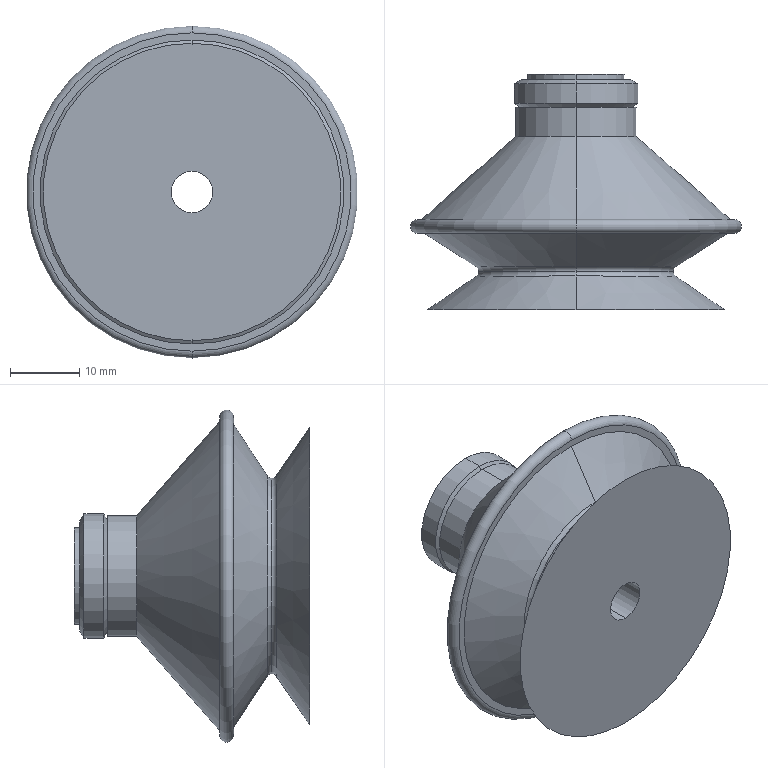Part | SolidWorks | features RefAxis 6, 3DProfileFeature 2, Revolution 1 | 1 solid | 30 faces | box 48 x 34 x 48 mm | volume 25361 mm3 | cone 10 | cylinder 8 | torus 6 | plane 6 | commonest cylinder face diameters 6 x2 14 x2 17.5 x2 18 x2
STEP:
#1=CARTESIAN_POINT('',(0.,6.152,14.498));
#2=VERTEX_POINT('',#1);
#3=CARTESIAN_POINT('',(0.,5.482,14.134));
#4=VERTEX_POINT('',#3);
#5=CARTESIAN_POINT('',(0.,5.482,14.934));
#6=DIRECTION('',(-1.,0.,0.));
#7=DIRECTION('',(0.,0.,1.));
#8=AXIS2_PLACEMENT_3D('',#5,#6,#7);
#9=CIRCLE('',#8,0.8);
#10=EDGE_CURVE('',#2,#4,#9,.T.);
#11=ORIENTED_EDGE('',*,*,#10,.T.);
#12=CARTESIAN_POINT('',(0.,5.482,-14.134));
#13=VERTEX_POINT('',#12);
#14=CARTESIAN_POINT('',(0.,5.482,0.));
#15=DIRECTION('',(0.,1.,0.));
#16=DIRECTION('',(0.,0.,1.));
#17=AXIS2_PLACEMENT_3D('',#14,#15,#16);
#18=CIRCLE('',#17,14.134);
#19=EDGE_CURVE('',#4,#13,#18,.T.);
#20=ORIENTED_EDGE('',*,*,#19,.T.);
#21=CARTESIAN_POINT('',(0.,6.152,-14.498));
#22=VERTEX_POINT('',#21);
#23=CARTESIAN_POINT('',(0.,5.482,-14.934));
#24=DIRECTION('',(1.,0.,0.));
#25=DIRECTION('',(0.,0.,-1.));
#26=AXIS2_PLACEMENT_3D('',#23,#24,#25);
#27=CIRCLE('',#26,0.8);
#28=EDGE_CURVE('',#22,#13,#27,.T.);
#29=ORIENTED_EDGE('',*,*,#28,.F.);
#30=CARTESIAN_POINT('',(0.,6.152,0.));
#31=DIRECTION('',(0.,1.,0.));
#32=DIRECTION('',(0.,0.,1.));
#33=AXIS2_PLACEMENT_3D('',#30,#31,#32);
#34=CIRCLE('',#33,14.498);
#35=EDGE_CURVE('',#2,#22,#34,.T.);
#36=ORIENTED_EDGE('',*,*,#35,.F.);
#37=EDGE_LOOP('',(#11,#20,#29,#36));
#38=FACE_OUTER_BOUND('',#37,.T.);
#39=CARTESIAN_POINT('',(0.,5.482,0.));
#40=DIRECTION('',(0.,1.,0.));
#41=DIRECTION('',(0.,0.,1.));
#42=AXIS2_PLACEMENT_3D('',#39,#40,#41);
#43=TOROIDAL_SURFACE('',#42,14.934,0.8);
#44=ADVANCED_FACE('',(#38),#43,.F.);
#45=ORIENTED_EDGE('',*,*,#28,.T.);
#46=CARTESIAN_POINT('',(0.,5.482,0.));
#47=DIRECTION('',(0.,1.,0.));
#48=DIRECTION('',(0.,0.,1.));
#49=AXIS2_PLACEMENT_3D('',#46,#47,#48);
#50=CIRCLE('',#49,14.134);
#51=EDGE_CURVE('',#13,#4,#50,.T.);
#52=ORIENTED_EDGE('',*,*,#51,.T.);
#53=ORIENTED_EDGE('',*,*,#10,.F.);
#54=CARTESIAN_POINT('',(0.,6.152,0.));
#55=DIRECTION('',(0.,1.,0.));
#56=DIRECTION('',(0.,0.,1.));
#57=AXIS2_PLACEMENT_3D('',#54,#55,#56);
#58=CIRCLE('',#57,14.498);
#59=EDGE_CURVE('',#22,#2,#58,.T.);
#60=ORIENTED_EDGE('',*,*,#59,.F.);
#61=EDGE_LOOP('',(#45,#52,#53,#60));
#62=FACE_OUTER_BOUND('',#61,.T.);
#63=CARTESIAN_POINT('',(0.,5.482,0.));
#64=DIRECTION('',(0.,1.,0.));
#65=DIRECTION('',(0.,0.,1.));
#66=AXIS2_PLACEMENT_3D('',#63,#64,#65);
#67=TOROIDAL_SURFACE('',#66,14.934,0.8);
#68=ADVANCED_FACE('',(#62),#67,.F.);
#69=CARTESIAN_POINT('',(0.,4.822,14.481));
#70=VERTEX_POINT('',#69);
#71=CARTESIAN_POINT('',(0.,4.822,-14.481));
#72=VERTEX_POINT('',#71);
#73=CARTESIAN_POINT('',(0.,4.822,0.));
#74=DIRECTION('',(0.,1.,0.));
#75=DIRECTION('',(0.,0.,1.));
#76=AXIS2_PLACEMENT_3D('',#73,#74,#75);
#77=CIRCLE('',#76,14.481);
#78=EDGE_CURVE('',#70,#72,#77,.T.);
#79=ORIENTED_EDGE('',*,*,#78,.F.);
#80=CARTESIAN_POINT('',(0.,0.,21.5));
#81=VERTEX_POINT('',#80);
#82=CARTESIAN_POINT('',(0.,0.,21.5));
#83=DIRECTION('',(0.,-0.5663,0.8242));
#84=VECTOR('',#83,1000.);
#85=LINE('',#82,#84);
#86=EDGE_CURVE('',#70,#81,#85,.T.);
#87=ORIENTED_EDGE('',*,*,#86,.T.);
#88=CARTESIAN_POINT('',(0.,0.,-21.5));
#89=VERTEX_POINT('',#88);
#90=CARTESIAN_POINT('',(0.,0.,0.));
#91=DIRECTION('',(0.,1.,0.));
#92=DIRECTION('',(0.,0.,1.));
#93=AXIS2_PLACEMENT_3D('',#90,#91,#92);
#94=CIRCLE('',#93,21.5);
#95=EDGE_CURVE('',#81,#89,#94,.T.);
#96=ORIENTED_EDGE('',*,*,#95,.T.);
#97=CARTESIAN_POINT('',(0.,0.,-21.5));
#98=DIRECTION('',(0.,-0.5663,-0.8242));
#99=VECTOR('',#98,1000.);
#100=LINE('',#97,#99);
#101=EDGE_CURVE('',#72,#89,#100,.T.);
#102=ORIENTED_EDGE('',*,*,#101,.F.);
#103=EDGE_LOOP('',(#79,#87,#96,#102));
#104=FACE_OUTER_BOUND('',#103,.T.);
#105=CARTESIAN_POINT('',(0.,0.,0.));
#106=DIRECTION('',(0.,-1.,0.));
#107=DIRECTION('',(0.,0.,-1.));
#108=AXIS2_PLACEMENT_3D('',#105,#106,#107);
#109=CONICAL_SURFACE('',#108,21.5,0.9688);
#110=ADVANCED_FACE('',(#104),#109,.T.);
#111=ORIENTED_EDGE('',*,*,#51,.F.);
#112=CARTESIAN_POINT('',(0.,5.482,-14.934));
#113=DIRECTION('',(1.,0.,0.));
#114=DIRECTION('',(0.,0.,-1.));
#115=AXIS2_PLACEMENT_3D('',#112,#113,#114);
#116=CIRCLE('',#115,0.8);
#117=EDGE_CURVE('',#13,#72,#116,.T.);
#118=ORIENTED_EDGE('',*,*,#117,.T.);
#119=CARTESIAN_POINT('',(0.,4.822,0.));
#120=DIRECTION('',(0.,1.,0.));
#121=DIRECTION('',(0.,0.,1.));
#122=AXIS2_PLACEMENT_3D('',#119,#120,#121);
#123=CIRCLE('',#122,14.481);
#124=EDGE_CURVE('',#72,#70,#123,.T.);
#125=ORIENTED_EDGE('',*,*,#124,.T.);
#126=CARTESIAN_POINT('',(0.,5.482,14.934));
#127=DIRECTION('',(-1.,0.,0.));
#128=DIRECTION('',(0.,0.,1.));
#129=AXIS2_PLACEMENT_3D('',#126,#127,#128);
#130=CIRCLE('',#129,0.8);
#131=EDGE_CURVE('',#4,#70,#130,.T.);
#132=ORIENTED_EDGE('',*,*,#131,.F.);
#133=EDGE_LOOP('',(#111,#118,#125,#132));
#134=FACE_OUTER_BOUND('',#133,.T.);
#135=CARTESIAN_POINT('',(0.,5.482,0.));
#136=DIRECTION('',(0.,1.,0.));
#137=DIRECTION('',(0.,0.,1.));
#138=AXIS2_PLACEMENT_3D('',#135,#136,#137);
#139=TOROIDAL_SURFACE('',#138,14.934,0.8);
#140=ADVANCED_FACE('',(#134),#139,.F.);
#141=ORIENTED_EDGE('',*,*,#35,.T.);
#142=CARTESIAN_POINT('',(0.,11.,-21.957));
#143=VERTEX_POINT('',#142);
#144=CARTESIAN_POINT('',(0.,6.152,-14.498));
#145=DIRECTION('',(0.,0.5449,-0.8385));
#146=VECTOR('',#145,1000.);
#147=LINE('',#144,#146);
#148=EDGE_CURVE('',#22,#143,#147,.T.);
#149=ORIENTED_EDGE('',*,*,#148,.T.);
#150=CARTESIAN_POINT('',(0.,11.,21.957));
#151=VERTEX_POINT('',#150);
#152=CARTESIAN_POINT('',(0.,11.,0.));
#153=DIRECTION('',(0.,1.,0.));
#154=DIRECTION('',(0.,0.,1.));
#155=AXIS2_PLACEMENT_3D('',#152,#153,#154);
#156=CIRCLE('',#155,21.957);
#157=EDGE_CURVE('',#151,#143,#156,.T.);
#158=ORIENTED_EDGE('',*,*,#157,.F.);
#159=CARTESIAN_POINT('',(0.,6.152,14.498));
#160=DIRECTION('',(0.,0.5449,0.8385));
#161=VECTOR('',#160,1000.);
#162=LINE('',#159,#161);
#163=EDGE_CURVE('',#2,#151,#162,.T.);
#164=ORIENTED_EDGE('',*,*,#163,.F.);
#165=EDGE_LOOP('',(#141,#149,#158,#164));
#166=FACE_OUTER_BOUND('',#165,.T.);
#167=CARTESIAN_POINT('',(0.,6.152,0.));
#168=DIRECTION('',(0.,1.,0.));
#169=DIRECTION('',(0.,0.,1.));
#170=AXIS2_PLACEMENT_3D('',#167,#168,#169);
#171=CONICAL_SURFACE('',#170,14.498,0.9945);
#172=ADVANCED_FACE('',(#166),#171,.T.);
#173=CARTESIAN_POINT('',(0.,11.,23.));
#174=VERTEX_POINT('',#173);
#175=CARTESIAN_POINT('',(0.,11.,-23.));
#176=VERTEX_POINT('',#175);
#177=CARTESIAN_POINT('',(0.,11.,0.));
#178=DIRECTION('',(0.,1.,0.));
#179=DIRECTION('',(0.,0.,1.));
#180=AXIS2_PLACEMENT_3D('',#177,#178,#179);
#181=CIRCLE('',#180,23.);
#182=EDGE_CURVE('',#174,#176,#181,.T.);
#183=ORIENTED_EDGE('',*,*,#182,.T.);
#184=CARTESIAN_POINT('',(0.,13.,-23.));
#185=VERTEX_POINT('',#184);
#186=CARTESIAN_POINT('',(0.,12.,-23.));
#187=DIRECTION('',(1.,0.,0.));
#188=DIRECTION('',(0.,0.,-1.));
#189=AXIS2_PLACEMENT_3D('',#186,#187,#188);
#190=CIRCLE('',#189,1.);
#191=EDGE_CURVE('',#176,#185,#190,.T.);
#192=ORIENTED_EDGE('',*,*,#191,.T.);
#193=CARTESIAN_POINT('',(0.,13.,23.));
#194=VERTEX_POINT('',#193);
#195=CARTESIAN_POINT('',(0.,13.,0.));
#196=DIRECTION('',(0.,1.,0.));
#197=DIRECTION('',(0.,0.,1.));
#198=AXIS2_PLACEMENT_3D('',#195,#196,#197);
#199=CIRCLE('',#198,23.);
#200=EDGE_CURVE('',#194,#185,#199,.T.);
#201=ORIENTED_EDGE('',*,*,#200,.F.);
#202=CARTESIAN_POINT('',(0.,12.,23.));
#203=DIRECTION('',(-1.,0.,0.));
#204=DIRECTION('',(0.,0.,1.));
#205=AXIS2_PLACEMENT_3D('',#202,#203,#204);
#206=CIRCLE('',#205,1.);
#207=EDGE_CURVE('',#174,#194,#206,.T.);
#208=ORIENTED_EDGE('',*,*,#207,.F.);
#209=EDGE_LOOP('',(#183,#192,#201,#208));
#210=FACE_OUTER_BOUND('',#209,.T.);
#211=CARTESIAN_POINT('',(0.,12.,0.));
#212=DIRECTION('',(0.,1.,0.));
#213=DIRECTION('',(0.,0.,1.));
#214=AXIS2_PLACEMENT_3D('',#211,#212,#213);
#215=TOROIDAL_SURFACE('',#214,23.,1.);
#216=ADVANCED_FACE('',(#210),#215,.T.);
#217=CARTESIAN_POINT('',(0.,25.,8.75));
#218=VERTEX_POINT('',#217);
#219=CARTESIAN_POINT('',(0.,25.,-8.75));
#220=VERTEX_POINT('',#219);
#221=CARTESIAN_POINT('',(0.,25.,0.));
#222=DIRECTION('',(0.,1.,0.));
#223=DIRECTION('',(0.,0.,1.));
#224=AXIS2_PLACEMENT_3D('',#221,#222,#223);
#225=CIRCLE('',#224,8.75);
#226=EDGE_CURVE('',#218,#220,#225,.T.);
#227=ORIENTED_EDGE('',*,*,#226,.F.);
#228=CARTESIAN_POINT('',(0.,13.,22.361));
#229=VERTEX_POINT('',#228);
#230=CARTESIAN_POINT('',(0.,13.,22.361));
#231=DIRECTION('',(0.,-0.6613,0.7501));
#232=VECTOR('',#231,1000.);
#233=LINE('',#230,#232);
#234=EDGE_CURVE('',#218,#229,#233,.T.);
#235=ORIENTED_EDGE('',*,*,#234,.T.);
#236=CARTESIAN_POINT('',(0.,13.,-22.361));
#237=VERTEX_POINT('',#236);
#238=CARTESIAN_POINT('',(0.,13.,0.));
#239=DIRECTION('',(0.,1.,0.));
#240=DIRECTION('',(0.,0.,1.));
#241=AXIS2_PLACEMENT_3D('',#238,#239,#240);
#242=CIRCLE('',#241,22.361);
#243=EDGE_CURVE('',#229,#237,#242,.T.);
#244=ORIENTED_EDGE('',*,*,#243,.T.);
#245=CARTESIAN_POINT('',(0.,13.,-22.361));
#246=DIRECTION('',(0.,-0.6613,-0.7501));
#247=VECTOR('',#246,1000.);
#248=LINE('',#245,#247);
#249=EDGE_CURVE('',#220,#237,#248,.T.);
#250=ORIENTED_EDGE('',*,*,#249,.F.);
#251=EDGE_LOOP('',(#227,#235,#244,#250));
#252=FACE_OUTER_BOUND('',#251,.T.);
#253=CARTESIAN_POINT('',(0.,13.,0.));
#254=DIRECTION('',(0.,-1.,0.));
#255=DIRECTION('',(0.,0.,-1.));
#256=AXIS2_PLACEMENT_3D('',#253,#254,#255);
#257=CONICAL_SURFACE('',#256,22.361,0.8482);
#258=ADVANCED_FACE('',(#252),#257,.T.);
#259=ORIENTED_EDGE('',*,*,#226,.T.);
#260=CARTESIAN_POINT('',(0.,29.2,-8.75));
#261=VERTEX_POINT('',#260);
#262=CARTESIAN_POINT('',(0.,0.,-8.75));
#263=DIRECTION('',(0.,1.,0.));
#264=VECTOR('',#263,1000.);
#265=LINE('',#262,#264);
#266=EDGE_CURVE('',#220,#261,#265,.T.);
#267=ORIENTED_EDGE('',*,*,#266,.T.);
#268=CARTESIAN_POINT('',(0.,29.2,8.75));
#269=VERTEX_POINT('',#268);
#270=CARTESIAN_POINT('',(0.,29.2,0.));
#271=DIRECTION('',(0.,1.,0.));
#272=DIRECTION('',(0.,0.,1.));
#273=AXIS2_PLACEMENT_3D('',#270,#271,#272);
#274=CIRCLE('',#273,8.75);
#275=EDGE_CURVE('',#269,#261,#274,.T.);
#276=ORIENTED_EDGE('',*,*,#275,.F.);
#277=CARTESIAN_POINT('',(0.,0.,8.75));
#278=DIRECTION('',(0.,1.,0.));
#279=VECTOR('',#278,1000.);
#280=LINE('',#277,#279);
#281=EDGE_CURVE('',#218,#269,#280,.T.);
#282=ORIENTED_EDGE('',*,*,#281,.F.);
#283=EDGE_LOOP('',(#259,#267,#276,#282));
#284=FACE_OUTER_BOUND('',#283,.T.);
#285=CARTESIAN_POINT('',(0.,0.,0.));
#286=DIRECTION('',(0.,1.,0.));
#287=DIRECTION('',(0.,0.,1.));
#288=AXIS2_PLACEMENT_3D('',#285,#286,#287);
#289=CYLINDRICAL_SURFACE('',#288,8.75);
#290=ADVANCED_FACE('',(#284),#289,.T.);
#291=CARTESIAN_POINT('',(0.,29.2,8.));
#292=VERTEX_POINT('',#291);
#293=CARTESIAN_POINT('',(0.,29.2,-8.));
#294=VERTEX_POINT('',#293);
#295=CARTESIAN_POINT('',(0.,29.2,0.));
#296=DIRECTION('',(0.,1.,0.));
#297=DIRECTION('',(0.,0.,1.));
#298=AXIS2_PLACEMENT_3D('',#295,#296,#297);
#299=CIRCLE('',#298,8.);
#300=EDGE_CURVE('',#292,#294,#299,.T.);
#301=ORIENTED_EDGE('',*,*,#300,.T.);
#302=CARTESIAN_POINT('',(0.,29.777,-9.));
#303=VERTEX_POINT('',#302);
#304=CARTESIAN_POINT('',(0.,29.2,-8.));
#305=DIRECTION('',(0.,0.5,-0.866));
#306=VECTOR('',#305,1000.);
#307=LINE('',#304,#306);
#308=EDGE_CURVE('',#294,#303,#307,.T.);
#309=ORIENTED_EDGE('',*,*,#308,.T.);
#310=CARTESIAN_POINT('',(0.,29.777,9.));
#311=VERTEX_POINT('',#310);
#312=CARTESIAN_POINT('',(0.,29.777,0.));
#313=DIRECTION('',(0.,1.,0.));
#314=DIRECTION('',(0.,0.,1.));
#315=AXIS2_PLACEMENT_3D('',#312,#313,#314);
#316=CIRCLE('',#315,9.);
#317=EDGE_CURVE('',#311,#303,#316,.T.);
#318=ORIENTED_EDGE('',*,*,#317,.F.);
#319=CARTESIAN_POINT('',(0.,29.2,8.));
#320=DIRECTION('',(0.,0.5,0.866));
#321=VECTOR('',#320,1000.);
#322=LINE('',#319,#321);
#323=EDGE_CURVE('',#292,#311,#322,.T.);
#324=ORIENTED_EDGE('',*,*,#323,.F.);
#325=EDGE_LOOP('',(#301,#309,#318,#324));
#326=FACE_OUTER_BOUND('',#325,.T.);
#327=CARTESIAN_POINT('',(0.,29.2,0.));
#328=DIRECTION('',(0.,1.,0.));
#329=DIRECTION('',(0.,0.,1.));
#330=AXIS2_PLACEMENT_3D('',#327,#328,#329);
#331=CONICAL_SURFACE('',#330,8.,1.047);
#332=ADVANCED_FACE('',(#326),#331,.T.);
#333=ORIENTED_EDGE('',*,*,#317,.T.);
#334=CARTESIAN_POINT('',(0.,32.623,-9.));
#335=VERTEX_POINT('',#334);
#336=CARTESIAN_POINT('',(0.,0.,-9.));
#337=DIRECTION('',(0.,1.,0.));
#338=VECTOR('',#337,1000.);
#339=LINE('',#336,#338);
#340=EDGE_CURVE('',#303,#335,#339,.T.);
#341=ORIENTED_EDGE('',*,*,#340,.T.);
#342=CARTESIAN_POINT('',(0.,32.623,9.));
#343=VERTEX_POINT('',#342);
#344=CARTESIAN_POINT('',(0.,32.623,0.));
#345=DIRECTION('',(0.,1.,0.));
#346=DIRECTION('',(0.,0.,1.));
#347=AXIS2_PLACEMENT_3D('',#344,#345,#346);
#348=CIRCLE('',#347,9.);
#349=EDGE_CURVE('',#343,#335,#348,.T.);
#350=ORIENTED_EDGE('',*,*,#349,.F.);
#351=CARTESIAN_POINT('',(0.,0.,9.));
#352=DIRECTION('',(0.,1.,0.));
#353=VECTOR('',#352,1000.);
#354=LINE('',#351,#353);
#355=EDGE_CURVE('',#311,#343,#354,.T.);
#356=ORIENTED_EDGE('',*,*,#355,.F.);
#357=EDGE_LOOP('',(#333,#341,#350,#356));
#358=FACE_OUTER_BOUND('',#357,.T.);
#359=CARTESIAN_POINT('',(0.,0.,0.));
#360=DIRECTION('',(0.,1.,0.));
#361=DIRECTION('',(0.,0.,1.));
#362=AXIS2_PLACEMENT_3D('',#359,#360,#361);
#363=CYLINDRICAL_SURFACE('',#362,9.);
#364=ADVANCED_FACE('',(#358),#363,.T.);
#365=CARTESIAN_POINT('',(0.,33.2,8.));
#366=VERTEX_POINT('',#365);
#367=CARTESIAN_POINT('',(0.,33.2,-8.));
#368=VERTEX_POINT('',#367);
#369=CARTESIAN_POINT('',(0.,33.2,0.));
#370=DIRECTION('',(0.,1.,0.));
#371=DIRECTION('',(0.,0.,1.));
#372=AXIS2_PLACEMENT_3D('',#369,#370,#371);
#373=CIRCLE('',#372,8.);
#374=EDGE_CURVE('',#366,#368,#373,.T.);
#375=ORIENTED_EDGE('',*,*,#374,.F.);
#376=CARTESIAN_POINT('',(0.,32.623,9.));
#377=DIRECTION('',(0.,-0.5,0.866));
#378=VECTOR('',#377,1000.);
#379=LINE('',#376,#378);
#380=EDGE_CURVE('',#366,#343,#379,.T.);
#381=ORIENTED_EDGE('',*,*,#380,.T.);
#382=ORIENTED_EDGE('',*,*,#349,.T.);
#383=CARTESIAN_POINT('',(0.,32.623,-9.));
#384=DIRECTION('',(0.,-0.5,-0.866));
#385=VECTOR('',#384,1000.);
#386=LINE('',#383,#385);
#387=EDGE_CURVE('',#368,#335,#386,.T.);
#388=ORIENTED_EDGE('',*,*,#387,.F.);
#389=EDGE_LOOP('',(#375,#381,#382,#388));
#390=FACE_OUTER_BOUND('',#389,.T.);
#391=CARTESIAN_POINT('',(0.,32.623,0.));
#392=DIRECTION('',(0.,-1.,0.));
#393=DIRECTION('',(0.,0.,-1.));
#394=AXIS2_PLACEMENT_3D('',#391,#392,#393);
#395=CONICAL_SURFACE('',#394,9.,1.047);
#396=ADVANCED_FACE('',(#390),#395,.T.);
#397=CARTESIAN_POINT('',(0.,33.2,7.));
#398=VERTEX_POINT('',#397);
#399=CARTESIAN_POINT('',(0.,33.2,-7.));
#400=VERTEX_POINT('',#399);
#401=CARTESIAN_POINT('',(0.,33.2,0.));
#402=DIRECTION('',(0.,1.,0.));
#403=DIRECTION('',(0.,0.,1.));
#404=AXIS2_PLACEMENT_3D('',#401,#402,#403);
#405=CIRCLE('',#404,7.);
#406=EDGE_CURVE('',#398,#400,#405,.T.);
#407=ORIENTED_EDGE('',*,*,#406,.T.);
#408=CARTESIAN_POINT('',(0.,34.,-7.));
#409=VERTEX_POINT('',#408);
#410=CARTESIAN_POINT('',(0.,0.,-7.));
#411=DIRECTION('',(0.,1.,0.));
#412=VECTOR('',#411,1000.);
#413=LINE('',#410,#412);
#414=EDGE_CURVE('',#400,#409,#413,.T.);
#415=ORIENTED_EDGE('',*,*,#414,.T.);
#416=CARTESIAN_POINT('',(0.,34.,7.));
#417=VERTEX_POINT('',#416);
#418=CARTESIAN_POINT('',(0.,34.,0.));
#419=DIRECTION('',(0.,1.,0.));
#420=DIRECTION('',(0.,0.,1.));
#421=AXIS2_PLACEMENT_3D('',#418,#419,#420);
#422=CIRCLE('',#421,7.);
#423=EDGE_CURVE('',#417,#409,#422,.T.);
#424=ORIENTED_EDGE('',*,*,#423,.F.);
#425=CARTESIAN_POINT('',(0.,0.,7.));
#426=DIRECTION('',(0.,1.,0.));
#427=VECTOR('',#426,1000.);
#428=LINE('',#425,#427);
#429=EDGE_CURVE('',#398,#417,#428,.T.);
#430=ORIENTED_EDGE('',*,*,#429,.F.);
#431=EDGE_LOOP('',(#407,#415,#424,#430));
#432=FACE_OUTER_BOUND('',#431,.T.);
#433=CARTESIAN_POINT('',(0.,0.,0.));
#434=DIRECTION('',(0.,1.,0.));
#435=DIRECTION('',(0.,0.,1.));
#436=AXIS2_PLACEMENT_3D('',#433,#434,#435);
#437=CYLINDRICAL_SURFACE('',#436,7.);
#438=ADVANCED_FACE('',(#432),#437,.T.);
#439=CARTESIAN_POINT('',(0.,0.,-3.));
#440=VERTEX_POINT('',#439);
#441=CARTESIAN_POINT('',(0.,0.,3.));
#442=VERTEX_POINT('',#441);
#443=CARTESIAN_POINT('',(0.,0.,0.));
#444=DIRECTION('',(0.,1.,0.));
#445=DIRECTION('',(0.,0.,1.));
#446=AXIS2_PLACEMENT_3D('',#443,#444,#445);
#447=CIRCLE('',#446,3.);
#448=EDGE_CURVE('',#440,#442,#447,.T.);
#449=ORIENTED_EDGE('',*,*,#448,.F.);
#450=CARTESIAN_POINT('',(0.,34.,-3.));
#451=VERTEX_POINT('',#450);
#452=CARTESIAN_POINT('',(0.,0.,-3.));
#453=DIRECTION('',(0.,1.,0.));
#454=VECTOR('',#453,1000.);
#455=LINE('',#452,#454);
#456=EDGE_CURVE('',#440,#451,#455,.T.);
#457=ORIENTED_EDGE('',*,*,#456,.T.);
#458=CARTESIAN_POINT('',(0.,34.,3.));
#459=VERTEX_POINT('',#458);
#460=CARTESIAN_POINT('',(0.,34.,0.));
#461=DIRECTION('',(0.,1.,0.));
#462=DIRECTION('',(0.,0.,1.));
#463=AXIS2_PLACEMENT_3D('',#460,#461,#462);
#464=CIRCLE('',#463,3.);
#465=EDGE_CURVE('',#451,#459,#464,.T.);
#466=ORIENTED_EDGE('',*,*,#465,.T.);
#467=CARTESIAN_POINT('',(0.,0.,3.));
#468=DIRECTION('',(0.,1.,0.));
#469=VECTOR('',#468,1000.);
#470=LINE('',#467,#469);
#471=EDGE_CURVE('',#442,#459,#470,.T.);
#472=ORIENTED_EDGE('',*,*,#471,.F.);
#473=EDGE_LOOP('',(#449,#457,#466,#472));
#474=FACE_OUTER_BOUND('',#473,.T.);
#475=CARTESIAN_POINT('',(0.,0.,0.));
#476=DIRECTION('',(0.,1.,0.));
#477=DIRECTION('',(0.,0.,1.));
#478=AXIS2_PLACEMENT_3D('',#475,#476,#477);
#479=CYLINDRICAL_SURFACE('',#478,3.);
#480=ADVANCED_FACE('',(#474),#479,.F.);
#481=ORIENTED_EDGE('',*,*,#456,.F.);
#482=CARTESIAN_POINT('',(0.,0.,0.));
#483=DIRECTION('',(0.,1.,0.));
#484=DIRECTION('',(0.,0.,1.));
#485=AXIS2_PLACEMENT_3D('',#482,#483,#484);
#486=CIRCLE('',#485,3.);
#487=EDGE_CURVE('',#442,#440,#486,.T.);
#488=ORIENTED_EDGE('',*,*,#487,.F.);
#489=ORIENTED_EDGE('',*,*,#471,.T.);
#490=CARTESIAN_POINT('',(0.,34.,0.));
#491=DIRECTION('',(0.,1.,0.));
#492=DIRECTION('',(0.,0.,1.));
#493=AXIS2_PLACEMENT_3D('',#490,#491,#492);
#494=CIRCLE('',#493,3.);
#495=EDGE_CURVE('',#459,#451,#494,.T.);
#496=ORIENTED_EDGE('',*,*,#495,.T.);
#497=EDGE_LOOP('',(#481,#488,#489,#496));
#498=FACE_OUTER_BOUND('',#497,.T.);
#499=CARTESIAN_POINT('',(0.,0.,0.));
#500=DIRECTION('',(0.,1.,0.));
#501=DIRECTION('',(0.,0.,1.));
#502=AXIS2_PLACEMENT_3D('',#499,#500,#501);
#503=CYLINDRICAL_SURFACE('',#502,3.);
#504=ADVANCED_FACE('',(#498),#503,.F.);
#505=ORIENTED_EDGE('',*,*,#495,.F.);
#506=ORIENTED_EDGE('',*,*,#465,.F.);
#507=EDGE_LOOP('',(#505,#506));
#508=FACE_BOUND('',#507,.T.);
#509=ORIENTED_EDGE('',*,*,#423,.T.);
#510=CARTESIAN_POINT('',(0.,34.,0.));
#511=DIRECTION('',(0.,1.,0.));
#512=DIRECTION('',(0.,0.,1.));
#513=AXIS2_PLACEMENT_3D('',#510,#511,#512);
#514=CIRCLE('',#513,7.);
#515=EDGE_CURVE('',#409,#417,#514,.T.);
#516=ORIENTED_EDGE('',*,*,#515,.T.);
#517=EDGE_LOOP('',(#509,#516));
#518=FACE_OUTER_BOUND('',#517,.T.);
#519=CARTESIAN_POINT('',(7.,34.,0.));
#520=DIRECTION('',(0.,-1.,0.));
#521=DIRECTION('',(0.,0.,-1.));
#522=AXIS2_PLACEMENT_3D('',#519,#520,#521);
#523=PLANE('',#522);
#524=ADVANCED_FACE('',(#508,#518),#523,.F.);
#525=ORIENTED_EDGE('',*,*,#414,.F.);
#526=CARTESIAN_POINT('',(0.,33.2,0.));
#527=DIRECTION('',(0.,1.,0.));
#528=DIRECTION('',(0.,0.,1.));
#529=AXIS2_PLACEMENT_3D('',#526,#527,#528);
#530=CIRCLE('',#529,7.);
#531=EDGE_CURVE('',#400,#398,#530,.T.);
#532=ORIENTED_EDGE('',*,*,#531,.T.);
#533=ORIENTED_EDGE('',*,*,#429,.T.);
#534=ORIENTED_EDGE('',*,*,#515,.F.);
#535=EDGE_LOOP('',(#525,#532,#533,#534));
#536=FACE_OUTER_BOUND('',#535,.T.);
#537=CARTESIAN_POINT('',(0.,0.,0.));
#538=DIRECTION('',(0.,1.,0.));
#539=DIRECTION('',(0.,0.,1.));
#540=AXIS2_PLACEMENT_3D('',#537,#538,#539);
#541=CYLINDRICAL_SURFACE('',#540,7.);
#542=ADVANCED_FACE('',(#536),#541,.T.);
#543=ORIENTED_EDGE('',*,*,#406,.F.);
#544=ORIENTED_EDGE('',*,*,#531,.F.);
#545=EDGE_LOOP('',(#543,#544));
#546=FACE_BOUND('',#545,.T.);
#547=CARTESIAN_POINT('',(0.,33.2,0.));
#548=DIRECTION('',(0.,1.,0.));
#549=DIRECTION('',(0.,0.,1.));
#550=AXIS2_PLACEMENT_3D('',#547,#548,#549);
#551=CIRCLE('',#550,8.);
#552=EDGE_CURVE('',#368,#366,#551,.T.);
#553=ORIENTED_EDGE('',*,*,#552,.T.);
#554=ORIENTED_EDGE('',*,*,#374,.T.);
#555=EDGE_LOOP('',(#553,#554));
#556=FACE_OUTER_BOUND('',#555,.T.);
#557=CARTESIAN_POINT('',(8.,33.2,0.));
#558=DIRECTION('',(0.,-1.,0.));
#559=DIRECTION('',(0.,0.,-1.));
#560=AXIS2_PLACEMENT_3D('',#557,#558,#559);
#561=PLANE('',#560);
#562=ADVANCED_FACE('',(#546,#556),#561,.F.);
#563=ORIENTED_EDGE('',*,*,#380,.F.);
#564=ORIENTED_EDGE('',*,*,#552,.F.);
#565=ORIENTED_EDGE('',*,*,#387,.T.);
#566=CARTESIAN_POINT('',(0.,32.623,0.));
#567=DIRECTION('',(0.,1.,0.));
#568=DIRECTION('',(0.,0.,1.));
#569=AXIS2_PLACEMENT_3D('',#566,#567,#568);
#570=CIRCLE('',#569,9.);
#571=EDGE_CURVE('',#335,#343,#570,.T.);
#572=ORIENTED_EDGE('',*,*,#571,.T.);
#573=EDGE_LOOP('',(#563,#564,#565,#572));
#574=FACE_OUTER_BOUND('',#573,.T.);
#575=CARTESIAN_POINT('',(0.,32.623,0.));
#576=DIRECTION('',(0.,-1.,0.));
#577=DIRECTION('',(0.,0.,-1.));
#578=AXIS2_PLACEMENT_3D('',#575,#576,#577);
#579=CONICAL_SURFACE('',#578,9.,1.047);
#580=ADVANCED_FACE('',(#574),#579,.T.);
#581=ORIENTED_EDGE('',*,*,#340,.F.);
#582=CARTESIAN_POINT('',(0.,29.777,0.));
#583=DIRECTION('',(0.,1.,0.));
#584=DIRECTION('',(0.,0.,1.));
#585=AXIS2_PLACEMENT_3D('',#582,#583,#584);
#586=CIRCLE('',#585,9.);
#587=EDGE_CURVE('',#303,#311,#586,.T.);
#588=ORIENTED_EDGE('',*,*,#587,.T.);
#589=ORIENTED_EDGE('',*,*,#355,.T.);
#590=ORIENTED_EDGE('',*,*,#571,.F.);
#591=EDGE_LOOP('',(#581,#588,#589,#590));
#592=FACE_OUTER_BOUND('',#591,.T.);
#593=CARTESIAN_POINT('',(0.,0.,0.));
#594=DIRECTION('',(0.,1.,0.));
#595=DIRECTION('',(0.,0.,1.));
#596=AXIS2_PLACEMENT_3D('',#593,#594,#595);
#597=CYLINDRICAL_SURFACE('',#596,9.);
#598=ADVANCED_FACE('',(#592),#597,.T.);
#599=ORIENTED_EDGE('',*,*,#308,.F.);
#600=CARTESIAN_POINT('',(0.,29.2,0.));
#601=DIRECTION('',(0.,1.,0.));
#602=DIRECTION('',(0.,0.,1.));
#603=AXIS2_PLACEMENT_3D('',#600,#601,#602);
#604=CIRCLE('',#603,8.);
#605=EDGE_CURVE('',#294,#292,#604,.T.);
#606=ORIENTED_EDGE('',*,*,#605,.T.);
#607=ORIENTED_EDGE('',*,*,#323,.T.);
#608=ORIENTED_EDGE('',*,*,#587,.F.);
#609=EDGE_LOOP('',(#599,#606,#607,#608));
#610=FACE_OUTER_BOUND('',#609,.T.);
#611=CARTESIAN_POINT('',(0.,29.2,0.));
#612=DIRECTION('',(0.,1.,0.));
#613=DIRECTION('',(0.,0.,1.));
#614=AXIS2_PLACEMENT_3D('',#611,#612,#613);
#615=CONICAL_SURFACE('',#614,8.,1.047);
#616=ADVANCED_FACE('',(#610),#615,.T.);
#617=ORIENTED_EDGE('',*,*,#300,.F.);
#618=ORIENTED_EDGE('',*,*,#605,.F.);
#619=EDGE_LOOP('',(#617,#618));
#620=FACE_BOUND('',#619,.T.);
#621=ORIENTED_EDGE('',*,*,#275,.T.);
#622=CARTESIAN_POINT('',(0.,29.2,0.));
#623=DIRECTION('',(0.,1.,0.));
#624=DIRECTION('',(0.,0.,1.));
#625=AXIS2_PLACEMENT_3D('',#622,#623,#624);
#626=CIRCLE('',#625,8.75);
#627=EDGE_CURVE('',#261,#269,#626,.T.);
#628=ORIENTED_EDGE('',*,*,#627,.T.);
#629=EDGE_LOOP('',(#621,#628));
#630=FACE_OUTER_BOUND('',#629,.T.);
#631=CARTESIAN_POINT('',(8.75,29.2,0.));
#632=DIRECTION('',(0.,-1.,0.));
#633=DIRECTION('',(0.,0.,-1.));
#634=AXIS2_PLACEMENT_3D('',#631,#632,#633);
#635=PLANE('',#634);
#636=ADVANCED_FACE('',(#620,#630),#635,.F.);
#637=ORIENTED_EDGE('',*,*,#266,.F.);
#638=CARTESIAN_POINT('',(0.,25.,0.));
#639=DIRECTION('',(0.,1.,0.));
#640=DIRECTION('',(0.,0.,1.));
#641=AXIS2_PLACEMENT_3D('',#638,#639,#640);
#642=CIRCLE('',#641,8.75);
#643=EDGE_CURVE('',#220,#218,#642,.T.);
#644=ORIENTED_EDGE('',*,*,#643,.T.);
#645=ORIENTED_EDGE('',*,*,#281,.T.);
#646=ORIENTED_EDGE('',*,*,#627,.F.);
#647=EDGE_LOOP('',(#637,#644,#645,#646));
#648=FACE_OUTER_BOUND('',#647,.T.);
#649=CARTESIAN_POINT('',(0.,0.,0.));
#650=DIRECTION('',(0.,1.,0.));
#651=DIRECTION('',(0.,0.,1.));
#652=AXIS2_PLACEMENT_3D('',#649,#650,#651);
#653=CYLINDRICAL_SURFACE('',#652,8.75);
#654=ADVANCED_FACE('',(#648),#653,.T.);
#655=ORIENTED_EDGE('',*,*,#234,.F.);
#656=ORIENTED_EDGE('',*,*,#643,.F.);
#657=ORIENTED_EDGE('',*,*,#249,.T.);
#658=CARTESIAN_POINT('',(0.,13.,0.));
#659=DIRECTION('',(0.,1.,0.));
#660=DIRECTION('',(0.,0.,1.));
#661=AXIS2_PLACEMENT_3D('',#658,#659,#660);
#662=CIRCLE('',#661,22.361);
#663=EDGE_CURVE('',#237,#229,#662,.T.);
#664=ORIENTED_EDGE('',*,*,#663,.T.);
#665=EDGE_LOOP('',(#655,#656,#657,#664));
#666=FACE_OUTER_BOUND('',#665,.T.);
#667=CARTESIAN_POINT('',(0.,13.,0.));
#668=DIRECTION('',(0.,-1.,0.));
#669=DIRECTION('',(0.,0.,-1.));
#670=AXIS2_PLACEMENT_3D('',#667,#668,#669);
#671=CONICAL_SURFACE('',#670,22.361,0.8482);
#672=ADVANCED_FACE('',(#666),#671,.T.);
#673=ORIENTED_EDGE('',*,*,#663,.F.);
#674=ORIENTED_EDGE('',*,*,#243,.F.);
#675=EDGE_LOOP('',(#673,#674));
#676=FACE_BOUND('',#675,.T.);
#677=ORIENTED_EDGE('',*,*,#200,.T.);
#678=CARTESIAN_POINT('',(0.,13.,0.));
#679=DIRECTION('',(0.,1.,0.));
#680=DIRECTION('',(0.,0.,1.));
#681=AXIS2_PLACEMENT_3D('',#678,#679,#680);
#682=CIRCLE('',#681,23.);
#683=EDGE_CURVE('',#185,#194,#682,.T.);
#684=ORIENTED_EDGE('',*,*,#683,.T.);
#685=EDGE_LOOP('',(#677,#684));
#686=FACE_OUTER_BOUND('',#685,.T.);
#687=CARTESIAN_POINT('',(23.,13.,0.));
#688=DIRECTION('',(0.,-1.,0.));
#689=DIRECTION('',(0.,0.,-1.));
#690=AXIS2_PLACEMENT_3D('',#687,#688,#689);
#691=PLANE('',#690);
#692=ADVANCED_FACE('',(#676,#686),#691,.F.);
#693=ORIENTED_EDGE('',*,*,#191,.F.);
#694=CARTESIAN_POINT('',(0.,11.,0.));
#695=DIRECTION('',(0.,1.,0.));
#696=DIRECTION('',(0.,0.,1.));
#697=AXIS2_PLACEMENT_3D('',#694,#695,#696);
#698=CIRCLE('',#697,23.);
#699=EDGE_CURVE('',#176,#174,#698,.T.);
#700=ORIENTED_EDGE('',*,*,#699,.T.);
#701=ORIENTED_EDGE('',*,*,#207,.T.);
#702=ORIENTED_EDGE('',*,*,#683,.F.);
#703=EDGE_LOOP('',(#693,#700,#701,#702));
#704=FACE_OUTER_BOUND('',#703,.T.);
#705=CARTESIAN_POINT('',(0.,12.,0.));
#706=DIRECTION('',(0.,1.,0.));
#707=DIRECTION('',(0.,0.,1.));
#708=AXIS2_PLACEMENT_3D('',#705,#706,#707);
#709=TOROIDAL_SURFACE('',#708,23.,1.);
#710=ADVANCED_FACE('',(#704),#709,.T.);
#711=ORIENTED_EDGE('',*,*,#182,.F.);
#712=ORIENTED_EDGE('',*,*,#699,.F.);
#713=EDGE_LOOP('',(#711,#712));
#714=FACE_OUTER_BOUND('',#713,.T.);
#715=ORIENTED_EDGE('',*,*,#157,.T.);
#716=CARTESIAN_POINT('',(0.,11.,0.));
#717=DIRECTION('',(0.,1.,0.));
#718=DIRECTION('',(0.,0.,1.));
#719=AXIS2_PLACEMENT_3D('',#716,#717,#718);
#720=CIRCLE('',#719,21.957);
#721=EDGE_CURVE('',#143,#151,#720,.T.);
#722=ORIENTED_EDGE('',*,*,#721,.T.);
#723=EDGE_LOOP('',(#715,#722));
#724=FACE_BOUND('',#723,.T.);
#725=CARTESIAN_POINT('',(21.957,11.,0.));
#726=DIRECTION('',(0.,1.,0.));
#727=DIRECTION('',(0.,0.,1.));
#728=AXIS2_PLACEMENT_3D('',#725,#726,#727);
#729=PLANE('',#728);
#730=ADVANCED_FACE('',(#714,#724),#729,.F.);
#731=ORIENTED_EDGE('',*,*,#148,.F.);
#732=ORIENTED_EDGE('',*,*,#59,.T.);
#733=ORIENTED_EDGE('',*,*,#163,.T.);
#734=ORIENTED_EDGE('',*,*,#721,.F.);
#735=EDGE_LOOP('',(#731,#732,#733,#734));
#736=FACE_OUTER_BOUND('',#735,.T.);
#737=CARTESIAN_POINT('',(0.,6.152,0.));
#738=DIRECTION('',(0.,1.,0.));
#739=DIRECTION('',(0.,0.,1.));
#740=AXIS2_PLACEMENT_3D('',#737,#738,#739);
#741=CONICAL_SURFACE('',#740,14.498,0.9945);
#742=ADVANCED_FACE('',(#736),#741,.T.);
#743=ORIENTED_EDGE('',*,*,#19,.F.);
#744=ORIENTED_EDGE('',*,*,#131,.T.);
#745=ORIENTED_EDGE('',*,*,#78,.T.);
#746=ORIENTED_EDGE('',*,*,#117,.F.);
#747=EDGE_LOOP('',(#743,#744,#745,#746));
#748=FACE_OUTER_BOUND('',#747,.T.);
#749=CARTESIAN_POINT('',(0.,5.482,0.));
#750=DIRECTION('',(0.,1.,0.));
#751=DIRECTION('',(0.,0.,1.));
#752=AXIS2_PLACEMENT_3D('',#749,#750,#751);
#753=TOROIDAL_SURFACE('',#752,14.934,0.8);
#754=ADVANCED_FACE('',(#748),#753,.F.);
#755=ORIENTED_EDGE('',*,*,#86,.F.);
#756=ORIENTED_EDGE('',*,*,#124,.F.);
#757=ORIENTED_EDGE('',*,*,#101,.T.);
#758=CARTESIAN_POINT('',(0.,0.,0.));
#759=DIRECTION('',(0.,1.,0.));
#760=DIRECTION('',(0.,0.,1.));
#761=AXIS2_PLACEMENT_3D('',#758,#759,#760);
#762=CIRCLE('',#761,21.5);
#763=EDGE_CURVE('',#89,#81,#762,.T.);
#764=ORIENTED_EDGE('',*,*,#763,.T.);
#765=EDGE_LOOP('',(#755,#756,#757,#764));
#766=FACE_OUTER_BOUND('',#765,.T.);
#767=CARTESIAN_POINT('',(0.,0.,0.));
#768=DIRECTION('',(0.,-1.,0.));
#769=DIRECTION('',(0.,0.,-1.));
#770=AXIS2_PLACEMENT_3D('',#767,#768,#769);
#771=CONICAL_SURFACE('',#770,21.5,0.9688);
#772=ADVANCED_FACE('',(#766),#771,.T.);
#773=ORIENTED_EDGE('',*,*,#763,.F.);
#774=ORIENTED_EDGE('',*,*,#95,.F.);
#775=EDGE_LOOP('',(#773,#774));
#776=FACE_OUTER_BOUND('',#775,.T.);
#777=ORIENTED_EDGE('',*,*,#487,.T.);
#778=ORIENTED_EDGE('',*,*,#448,.T.);
#779=EDGE_LOOP('',(#777,#778));
#780=FACE_BOUND('',#779,.T.);
#781=CARTESIAN_POINT('',(3.,0.,0.));
#782=DIRECTION('',(0.,1.,0.));
#783=DIRECTION('',(0.,0.,1.));
#784=AXIS2_PLACEMENT_3D('',#781,#782,#783);
#785=PLANE('',#784);
#786=ADVANCED_FACE('',(#776,#780),#785,.F.);
#787=CLOSED_SHELL('',(#44,#68,#110,#140,#172,#216,#258,#290,#332,#364,#396,#438,#480,#504,#524,#542,#562,#580,#598,#616,#636,#654,#672,#692,#710,#730,#742,#754,#772,#786));
#788=MANIFOLD_SOLID_BREP('',#787);
#789=CARTESIAN_POINT('',(0.,0.,0.));
#790=DIRECTION('',(0.,0.,1.));
#791=DIRECTION('',(1.,0.,0.));
#792=AXIS2_PLACEMENT_3D('',#789,#790,#791);
#793=(LENGTH_UNIT()NAMED_UNIT(*)SI_UNIT(.MILLI.,.METRE.));
#794=UNCERTAINTY_MEASURE_WITH_UNIT(LENGTH_MEASURE(0.00001),#793,'','');
#795=(NAMED_UNIT(*)PLANE_ANGLE_UNIT()SI_UNIT($,.RADIAN.));
#796=(NAMED_UNIT(*)SI_UNIT($,.STERADIAN.)SOLID_ANGLE_UNIT());
#797=(GEOMETRIC_REPRESENTATION_CONTEXT(3)GLOBAL_UNCERTAINTY_ASSIGNED_CONTEXT((#794))GLOBAL_UNIT_ASSIGNED_CONTEXT((#793,#795,#796))REPRESENTATION_CONTEXT('',''));
#798=ADVANCED_BREP_SHAPE_REPRESENTATION('',(#788,#792),#797);